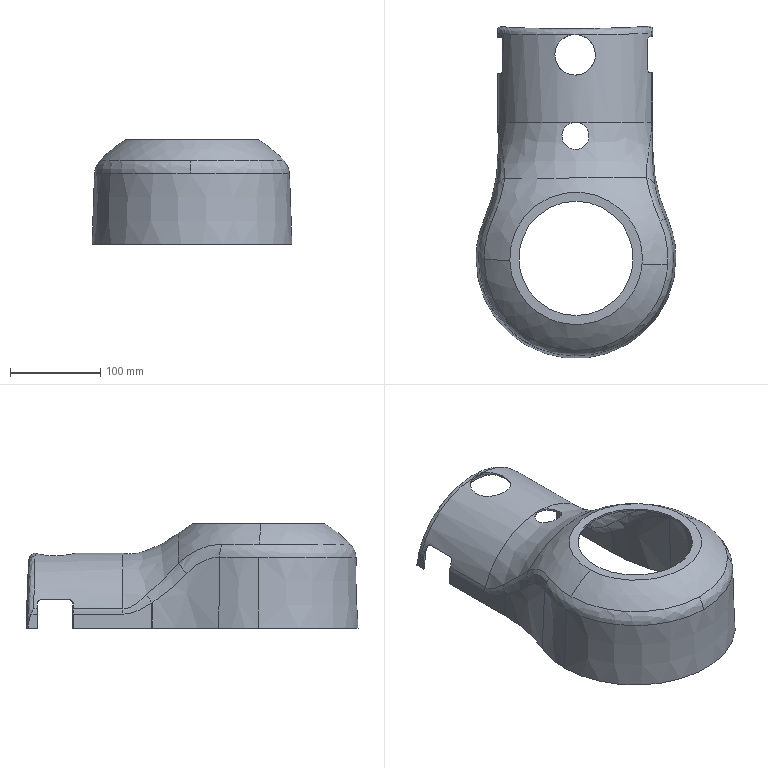Part | SolidWorks | features BaseBody 1 | 1 solid | 88 faces | box 221.968 x 369.168 x 116.123 mm | volume 238277 mm3 | spline 26 | plane 24 | cylinder 21 | cone 17 | commonest cylinder face diameters 10 x4 40 x4 44 x4 30 x2 45 x2 127 x2